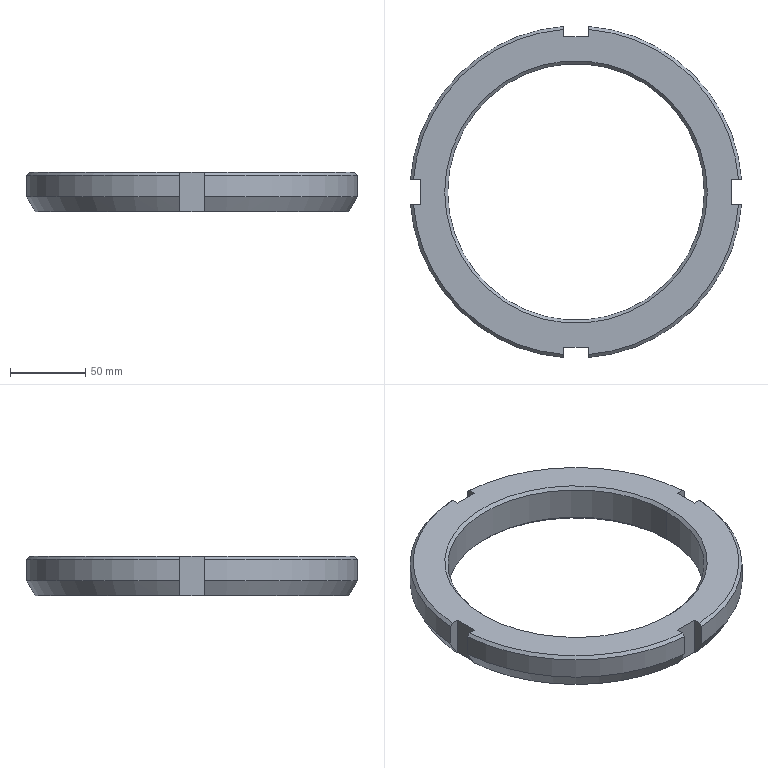Part | SolidWorks | features Chamfer 3, ICE 2, Extrusion 1 | 1 solid | 32 faces | box 219.417 x 219.417 x 26 mm | volume 365558 mm3 | plane 14 | cone 12 | cylinder 6 | commonest cylinder face diameters 220 x4 170 x2
STEP:
#1=CARTESIAN_POINT('',(85.,0.,2.));
#2=VERTEX_POINT('',#1);
#3=CARTESIAN_POINT('',(-85.,0.,2.));
#4=VERTEX_POINT('',#3);
#5=CARTESIAN_POINT('',(0.,0.,2.));
#6=DIRECTION('',(0.,0.,-1.));
#7=DIRECTION('',(1.,0.,0.));
#8=AXIS2_PLACEMENT_3D('',#5,#6,#7);
#9=CIRCLE('',#8,85.);
#10=EDGE_CURVE('',#2,#4,#9,.T.);
#11=ORIENTED_EDGE('',*,*,#10,.F.);
#12=CARTESIAN_POINT('',(87.,0.,0.));
#13=VERTEX_POINT('',#12);
#14=CARTESIAN_POINT('',(85.,0.,2.));
#15=DIRECTION('',(0.7071,0.,-0.7071));
#16=VECTOR('',#15,1000.);
#17=LINE('',#14,#16);
#18=EDGE_CURVE('',#2,#13,#17,.T.);
#19=ORIENTED_EDGE('',*,*,#18,.T.);
#20=CARTESIAN_POINT('',(-87.,0.,0.));
#21=VERTEX_POINT('',#20);
#22=CARTESIAN_POINT('',(0.,0.,0.));
#23=DIRECTION('',(0.,0.,1.));
#24=DIRECTION('',(1.,0.,0.));
#25=AXIS2_PLACEMENT_3D('',#22,#23,#24);
#26=CIRCLE('',#25,87.);
#27=EDGE_CURVE('',#21,#13,#26,.T.);
#28=ORIENTED_EDGE('',*,*,#27,.F.);
#29=CARTESIAN_POINT('',(-85.,0.,2.));
#30=DIRECTION('',(-0.7071,0.,-0.7071));
#31=VECTOR('',#30,1000.);
#32=LINE('',#29,#31);
#33=EDGE_CURVE('',#4,#21,#32,.T.);
#34=ORIENTED_EDGE('',*,*,#33,.F.);
#35=EDGE_LOOP('',(#11,#19,#28,#34));
#36=FACE_OUTER_BOUND('',#35,.T.);
#37=CARTESIAN_POINT('',(0.,0.,2.));
#38=DIRECTION('',(0.,0.,-1.));
#39=DIRECTION('',(-1.,0.,0.));
#40=AXIS2_PLACEMENT_3D('',#37,#38,#39);
#41=CONICAL_SURFACE('',#40,85.,0.7854);
#42=ADVANCED_FACE('',(#36),#41,.F.);
#43=CARTESIAN_POINT('',(-85.,0.,24.));
#44=VERTEX_POINT('',#43);
#45=CARTESIAN_POINT('',(85.,0.,24.));
#46=VERTEX_POINT('',#45);
#47=CARTESIAN_POINT('',(0.,0.,24.));
#48=DIRECTION('',(0.,0.,1.));
#49=DIRECTION('',(1.,0.,0.));
#50=AXIS2_PLACEMENT_3D('',#47,#48,#49);
#51=CIRCLE('',#50,85.);
#52=EDGE_CURVE('',#44,#46,#51,.T.);
#53=ORIENTED_EDGE('',*,*,#52,.F.);
#54=CARTESIAN_POINT('',(-87.,0.,26.));
#55=VERTEX_POINT('',#54);
#56=CARTESIAN_POINT('',(-87.,0.,26.));
#57=DIRECTION('',(-0.7071,0.,0.7071));
#58=VECTOR('',#57,1000.);
#59=LINE('',#56,#58);
#60=EDGE_CURVE('',#44,#55,#59,.T.);
#61=ORIENTED_EDGE('',*,*,#60,.T.);
#62=CARTESIAN_POINT('',(87.,0.,26.));
#63=VERTEX_POINT('',#62);
#64=CARTESIAN_POINT('',(0.,0.,26.));
#65=DIRECTION('',(0.,0.,-1.));
#66=DIRECTION('',(1.,0.,0.));
#67=AXIS2_PLACEMENT_3D('',#64,#65,#66);
#68=CIRCLE('',#67,87.);
#69=EDGE_CURVE('',#63,#55,#68,.T.);
#70=ORIENTED_EDGE('',*,*,#69,.F.);
#71=CARTESIAN_POINT('',(87.,0.,26.));
#72=DIRECTION('',(0.7071,0.,0.7071));
#73=VECTOR('',#72,1000.);
#74=LINE('',#71,#73);
#75=EDGE_CURVE('',#46,#63,#74,.T.);
#76=ORIENTED_EDGE('',*,*,#75,.F.);
#77=EDGE_LOOP('',(#53,#61,#70,#76));
#78=FACE_OUTER_BOUND('',#77,.T.);
#79=CARTESIAN_POINT('',(0.,0.,26.));
#80=DIRECTION('',(0.,0.,1.));
#81=DIRECTION('',(1.,0.,0.));
#82=AXIS2_PLACEMENT_3D('',#79,#80,#81);
#83=CONICAL_SURFACE('',#82,87.,0.7854);
#84=ADVANCED_FACE('',(#78),#83,.F.);
#85=ORIENTED_EDGE('',*,*,#52,.T.);
#86=CARTESIAN_POINT('',(85.,0.,26.));
#87=DIRECTION('',(0.,0.,-1.));
#88=VECTOR('',#87,1000.);
#89=LINE('',#86,#88);
#90=EDGE_CURVE('',#46,#2,#89,.T.);
#91=ORIENTED_EDGE('',*,*,#90,.T.);
#92=ORIENTED_EDGE('',*,*,#10,.T.);
#93=CARTESIAN_POINT('',(-85.,0.,26.));
#94=DIRECTION('',(0.,0.,-1.));
#95=VECTOR('',#94,1000.);
#96=LINE('',#93,#95);
#97=EDGE_CURVE('',#44,#4,#96,.T.);
#98=ORIENTED_EDGE('',*,*,#97,.F.);
#99=EDGE_LOOP('',(#85,#91,#92,#98));
#100=FACE_OUTER_BOUND('',#99,.T.);
#101=CARTESIAN_POINT('',(0.,0.,26.));
#102=DIRECTION('',(0.,0.,-1.));
#103=DIRECTION('',(-1.,0.,0.));
#104=AXIS2_PLACEMENT_3D('',#101,#102,#103);
#105=CYLINDRICAL_SURFACE('',#104,85.);
#106=ADVANCED_FACE('',(#100),#105,.F.);
#107=CARTESIAN_POINT('',(8.,-109.709,24.));
#108=VERTEX_POINT('',#107);
#109=CARTESIAN_POINT('',(8.,-109.709,10.));
#110=VERTEX_POINT('',#109);
#111=CARTESIAN_POINT('',(8.,-109.709,26.));
#112=DIRECTION('',(0.,0.,-1.));
#113=VECTOR('',#112,1000.);
#114=LINE('',#111,#113);
#115=EDGE_CURVE('',#108,#110,#114,.T.);
#116=ORIENTED_EDGE('',*,*,#115,.T.);
#117=CARTESIAN_POINT('',(109.709,-8.,10.));
#118=VERTEX_POINT('',#117);
#119=CARTESIAN_POINT('',(0.,0.,10.));
#120=DIRECTION('',(0.,0.,1.));
#121=DIRECTION('',(1.,0.,0.));
#122=AXIS2_PLACEMENT_3D('',#119,#120,#121);
#123=CIRCLE('',#122,110.);
#124=EDGE_CURVE('',#110,#118,#123,.T.);
#125=ORIENTED_EDGE('',*,*,#124,.T.);
#126=CARTESIAN_POINT('',(109.709,-8.,24.));
#127=VERTEX_POINT('',#126);
#128=CARTESIAN_POINT('',(109.709,-8.,26.));
#129=DIRECTION('',(0.,0.,1.));
#130=VECTOR('',#129,1000.);
#131=LINE('',#128,#130);
#132=EDGE_CURVE('',#118,#127,#131,.T.);
#133=ORIENTED_EDGE('',*,*,#132,.T.);
#134=CARTESIAN_POINT('',(0.,0.,24.));
#135=DIRECTION('',(0.,0.,-1.));
#136=DIRECTION('',(1.,0.,0.));
#137=AXIS2_PLACEMENT_3D('',#134,#135,#136);
#138=CIRCLE('',#137,110.);
#139=EDGE_CURVE('',#127,#108,#138,.T.);
#140=ORIENTED_EDGE('',*,*,#139,.T.);
#141=EDGE_LOOP('',(#116,#125,#133,#140));
#142=FACE_OUTER_BOUND('',#141,.T.);
#143=CARTESIAN_POINT('',(0.,0.,26.));
#144=DIRECTION('',(0.,0.,-1.));
#145=DIRECTION('',(-1.,0.,0.));
#146=AXIS2_PLACEMENT_3D('',#143,#144,#145);
#147=CYLINDRICAL_SURFACE('',#146,110.);
#148=ADVANCED_FACE('',(#142),#147,.T.);
#149=CARTESIAN_POINT('',(-8.,109.709,24.));
#150=VERTEX_POINT('',#149);
#151=CARTESIAN_POINT('',(-8.,109.709,10.));
#152=VERTEX_POINT('',#151);
#153=CARTESIAN_POINT('',(-8.,109.709,26.));
#154=DIRECTION('',(0.,0.,-1.));
#155=VECTOR('',#154,1000.);
#156=LINE('',#153,#155);
#157=EDGE_CURVE('',#150,#152,#156,.T.);
#158=ORIENTED_EDGE('',*,*,#157,.T.);
#159=CARTESIAN_POINT('',(-109.709,8.,10.));
#160=VERTEX_POINT('',#159);
#161=CARTESIAN_POINT('',(0.,0.,10.));
#162=DIRECTION('',(0.,0.,1.));
#163=DIRECTION('',(1.,0.,0.));
#164=AXIS2_PLACEMENT_3D('',#161,#162,#163);
#165=CIRCLE('',#164,110.);
#166=EDGE_CURVE('',#152,#160,#165,.T.);
#167=ORIENTED_EDGE('',*,*,#166,.T.);
#168=CARTESIAN_POINT('',(-109.709,8.,24.));
#169=VERTEX_POINT('',#168);
#170=CARTESIAN_POINT('',(-109.709,8.,26.));
#171=DIRECTION('',(0.,0.,1.));
#172=VECTOR('',#171,1000.);
#173=LINE('',#170,#172);
#174=EDGE_CURVE('',#160,#169,#173,.T.);
#175=ORIENTED_EDGE('',*,*,#174,.T.);
#176=CARTESIAN_POINT('',(0.,0.,24.));
#177=DIRECTION('',(0.,0.,-1.));
#178=DIRECTION('',(1.,0.,0.));
#179=AXIS2_PLACEMENT_3D('',#176,#177,#178);
#180=CIRCLE('',#179,110.);
#181=EDGE_CURVE('',#169,#150,#180,.T.);
#182=ORIENTED_EDGE('',*,*,#181,.T.);
#183=EDGE_LOOP('',(#158,#167,#175,#182));
#184=FACE_OUTER_BOUND('',#183,.T.);
#185=CARTESIAN_POINT('',(0.,0.,26.));
#186=DIRECTION('',(0.,0.,-1.));
#187=DIRECTION('',(-1.,0.,0.));
#188=AXIS2_PLACEMENT_3D('',#185,#186,#187);
#189=CYLINDRICAL_SURFACE('',#188,110.);
#190=ADVANCED_FACE('',(#184),#189,.T.);
#191=CARTESIAN_POINT('',(-109.709,-8.,24.));
#192=VERTEX_POINT('',#191);
#193=CARTESIAN_POINT('',(-109.709,-8.,10.));
#194=VERTEX_POINT('',#193);
#195=CARTESIAN_POINT('',(-109.709,-8.,26.));
#196=DIRECTION('',(0.,0.,-1.));
#197=VECTOR('',#196,1000.);
#198=LINE('',#195,#197);
#199=EDGE_CURVE('',#192,#194,#198,.T.);
#200=ORIENTED_EDGE('',*,*,#199,.T.);
#201=CARTESIAN_POINT('',(-8.,-109.709,10.));
#202=VERTEX_POINT('',#201);
#203=CARTESIAN_POINT('',(0.,0.,10.));
#204=DIRECTION('',(0.,0.,1.));
#205=DIRECTION('',(1.,0.,0.));
#206=AXIS2_PLACEMENT_3D('',#203,#204,#205);
#207=CIRCLE('',#206,110.);
#208=EDGE_CURVE('',#194,#202,#207,.T.);
#209=ORIENTED_EDGE('',*,*,#208,.T.);
#210=CARTESIAN_POINT('',(-8.,-109.709,24.));
#211=VERTEX_POINT('',#210);
#212=CARTESIAN_POINT('',(-8.,-109.709,26.));
#213=DIRECTION('',(0.,0.,1.));
#214=VECTOR('',#213,1000.);
#215=LINE('',#212,#214);
#216=EDGE_CURVE('',#202,#211,#215,.T.);
#217=ORIENTED_EDGE('',*,*,#216,.T.);
#218=CARTESIAN_POINT('',(0.,0.,24.));
#219=DIRECTION('',(0.,0.,-1.));
#220=DIRECTION('',(1.,0.,0.));
#221=AXIS2_PLACEMENT_3D('',#218,#219,#220);
#222=CIRCLE('',#221,110.);
#223=EDGE_CURVE('',#211,#192,#222,.T.);
#224=ORIENTED_EDGE('',*,*,#223,.T.);
#225=EDGE_LOOP('',(#200,#209,#217,#224));
#226=FACE_OUTER_BOUND('',#225,.T.);
#227=CARTESIAN_POINT('',(0.,0.,26.));
#228=DIRECTION('',(0.,0.,-1.));
#229=DIRECTION('',(-1.,0.,0.));
#230=AXIS2_PLACEMENT_3D('',#227,#228,#229);
#231=CYLINDRICAL_SURFACE('',#230,110.);
#232=ADVANCED_FACE('',(#226),#231,.T.);
#233=CARTESIAN_POINT('',(109.709,8.,24.));
#234=VERTEX_POINT('',#233);
#235=CARTESIAN_POINT('',(109.709,8.,10.));
#236=VERTEX_POINT('',#235);
#237=CARTESIAN_POINT('',(109.709,8.,26.));
#238=DIRECTION('',(0.,0.,-1.));
#239=VECTOR('',#238,1000.);
#240=LINE('',#237,#239);
#241=EDGE_CURVE('',#234,#236,#240,.T.);
#242=ORIENTED_EDGE('',*,*,#241,.T.);
#243=CARTESIAN_POINT('',(8.,109.709,10.));
#244=VERTEX_POINT('',#243);
#245=CARTESIAN_POINT('',(0.,0.,10.));
#246=DIRECTION('',(0.,0.,1.));
#247=DIRECTION('',(1.,0.,0.));
#248=AXIS2_PLACEMENT_3D('',#245,#246,#247);
#249=CIRCLE('',#248,110.);
#250=EDGE_CURVE('',#236,#244,#249,.T.);
#251=ORIENTED_EDGE('',*,*,#250,.T.);
#252=CARTESIAN_POINT('',(8.,109.709,24.));
#253=VERTEX_POINT('',#252);
#254=CARTESIAN_POINT('',(8.,109.709,26.));
#255=DIRECTION('',(0.,0.,1.));
#256=VECTOR('',#255,1000.);
#257=LINE('',#254,#256);
#258=EDGE_CURVE('',#244,#253,#257,.T.);
#259=ORIENTED_EDGE('',*,*,#258,.T.);
#260=CARTESIAN_POINT('',(0.,0.,24.));
#261=DIRECTION('',(0.,0.,-1.));
#262=DIRECTION('',(1.,0.,0.));
#263=AXIS2_PLACEMENT_3D('',#260,#261,#262);
#264=CIRCLE('',#263,110.);
#265=EDGE_CURVE('',#253,#234,#264,.T.);
#266=ORIENTED_EDGE('',*,*,#265,.T.);
#267=EDGE_LOOP('',(#242,#251,#259,#266));
#268=FACE_OUTER_BOUND('',#267,.T.);
#269=CARTESIAN_POINT('',(0.,0.,26.));
#270=DIRECTION('',(0.,0.,-1.));
#271=DIRECTION('',(-1.,0.,0.));
#272=AXIS2_PLACEMENT_3D('',#269,#270,#271);
#273=CYLINDRICAL_SURFACE('',#272,110.);
#274=ADVANCED_FACE('',(#268),#273,.T.);
#275=ORIENTED_EDGE('',*,*,#69,.T.);
#276=CARTESIAN_POINT('',(0.,0.,26.));
#277=DIRECTION('',(0.,0.,-1.));
#278=DIRECTION('',(1.,0.,0.));
#279=AXIS2_PLACEMENT_3D('',#276,#277,#278);
#280=CIRCLE('',#279,87.);
#281=EDGE_CURVE('',#55,#63,#280,.T.);
#282=ORIENTED_EDGE('',*,*,#281,.T.);
#283=EDGE_LOOP('',(#275,#282));
#284=FACE_BOUND('',#283,.T.);
#285=CARTESIAN_POINT('',(8.,-107.703,26.));
#286=VERTEX_POINT('',#285);
#287=CARTESIAN_POINT('',(8.,-103.,26.));
#288=VERTEX_POINT('',#287);
#289=CARTESIAN_POINT('',(8.,-103.,26.));
#290=DIRECTION('',(0.,1.,0.));
#291=VECTOR('',#290,1000.);
#292=LINE('',#289,#291);
#293=EDGE_CURVE('',#286,#288,#292,.T.);
#294=ORIENTED_EDGE('',*,*,#293,.F.);
#295=CARTESIAN_POINT('',(107.703,-8.,26.));
#296=VERTEX_POINT('',#295);
#297=CARTESIAN_POINT('',(0.,0.,26.));
#298=DIRECTION('',(0.,0.,1.));
#299=DIRECTION('',(1.,0.,0.));
#300=AXIS2_PLACEMENT_3D('',#297,#298,#299);
#301=CIRCLE('',#300,108.);
#302=EDGE_CURVE('',#286,#296,#301,.T.);
#303=ORIENTED_EDGE('',*,*,#302,.T.);
#304=CARTESIAN_POINT('',(103.,-8.,26.));
#305=VERTEX_POINT('',#304);
#306=CARTESIAN_POINT('',(103.,-8.,26.));
#307=DIRECTION('',(1.,0.,0.));
#308=VECTOR('',#307,1000.);
#309=LINE('',#306,#308);
#310=EDGE_CURVE('',#305,#296,#309,.T.);
#311=ORIENTED_EDGE('',*,*,#310,.F.);
#312=CARTESIAN_POINT('',(103.,8.,26.));
#313=VERTEX_POINT('',#312);
#314=CARTESIAN_POINT('',(103.,8.,26.));
#315=DIRECTION('',(0.,-1.,0.));
#316=VECTOR('',#315,1000.);
#317=LINE('',#314,#316);
#318=EDGE_CURVE('',#313,#305,#317,.T.);
#319=ORIENTED_EDGE('',*,*,#318,.F.);
#320=CARTESIAN_POINT('',(107.703,8.,26.));
#321=VERTEX_POINT('',#320);
#322=CARTESIAN_POINT('',(103.,8.,26.));
#323=DIRECTION('',(-1.,0.,0.));
#324=VECTOR('',#323,1000.);
#325=LINE('',#322,#324);
#326=EDGE_CURVE('',#321,#313,#325,.T.);
#327=ORIENTED_EDGE('',*,*,#326,.F.);
#328=CARTESIAN_POINT('',(8.,107.703,26.));
#329=VERTEX_POINT('',#328);
#330=CARTESIAN_POINT('',(0.,0.,26.));
#331=DIRECTION('',(0.,0.,1.));
#332=DIRECTION('',(1.,0.,0.));
#333=AXIS2_PLACEMENT_3D('',#330,#331,#332);
#334=CIRCLE('',#333,108.);
#335=EDGE_CURVE('',#321,#329,#334,.T.);
#336=ORIENTED_EDGE('',*,*,#335,.T.);
#337=CARTESIAN_POINT('',(8.,103.,26.));
#338=VERTEX_POINT('',#337);
#339=CARTESIAN_POINT('',(8.,109.954,26.));
#340=DIRECTION('',(0.,1.,0.));
#341=VECTOR('',#340,1000.);
#342=LINE('',#339,#341);
#343=EDGE_CURVE('',#338,#329,#342,.T.);
#344=ORIENTED_EDGE('',*,*,#343,.F.);
#345=CARTESIAN_POINT('',(-8.,103.,26.));
#346=VERTEX_POINT('',#345);
#347=CARTESIAN_POINT('',(-8.,103.,26.));
#348=DIRECTION('',(1.,0.,0.));
#349=VECTOR('',#348,1000.);
#350=LINE('',#347,#349);
#351=EDGE_CURVE('',#346,#338,#350,.T.);
#352=ORIENTED_EDGE('',*,*,#351,.F.);
#353=CARTESIAN_POINT('',(-8.,107.703,26.));
#354=VERTEX_POINT('',#353);
#355=CARTESIAN_POINT('',(-8.,109.954,26.));
#356=DIRECTION('',(0.,-1.,0.));
#357=VECTOR('',#356,1000.);
#358=LINE('',#355,#357);
#359=EDGE_CURVE('',#354,#346,#358,.T.);
#360=ORIENTED_EDGE('',*,*,#359,.F.);
#361=CARTESIAN_POINT('',(-107.703,8.,26.));
#362=VERTEX_POINT('',#361);
#363=CARTESIAN_POINT('',(0.,0.,26.));
#364=DIRECTION('',(0.,0.,1.));
#365=DIRECTION('',(1.,0.,0.));
#366=AXIS2_PLACEMENT_3D('',#363,#364,#365);
#367=CIRCLE('',#366,108.);
#368=EDGE_CURVE('',#354,#362,#367,.T.);
#369=ORIENTED_EDGE('',*,*,#368,.T.);
#370=CARTESIAN_POINT('',(-103.,8.,26.));
#371=VERTEX_POINT('',#370);
#372=CARTESIAN_POINT('',(-109.954,8.,26.));
#373=DIRECTION('',(-1.,0.,0.));
#374=VECTOR('',#373,1000.);
#375=LINE('',#372,#374);
#376=EDGE_CURVE('',#371,#362,#375,.T.);
#377=ORIENTED_EDGE('',*,*,#376,.F.);
#378=CARTESIAN_POINT('',(-103.,-8.,26.));
#379=VERTEX_POINT('',#378);
#380=CARTESIAN_POINT('',(-103.,8.,26.));
#381=DIRECTION('',(0.,1.,0.));
#382=VECTOR('',#381,1000.);
#383=LINE('',#380,#382);
#384=EDGE_CURVE('',#379,#371,#383,.T.);
#385=ORIENTED_EDGE('',*,*,#384,.F.);
#386=CARTESIAN_POINT('',(-107.703,-8.,26.));
#387=VERTEX_POINT('',#386);
#388=CARTESIAN_POINT('',(-109.954,-8.,26.));
#389=DIRECTION('',(1.,0.,0.));
#390=VECTOR('',#389,1000.);
#391=LINE('',#388,#390);
#392=EDGE_CURVE('',#387,#379,#391,.T.);
#393=ORIENTED_EDGE('',*,*,#392,.F.);
#394=CARTESIAN_POINT('',(-8.,-107.703,26.));
#395=VERTEX_POINT('',#394);
#396=CARTESIAN_POINT('',(0.,0.,26.));
#397=DIRECTION('',(0.,0.,1.));
#398=DIRECTION('',(1.,0.,0.));
#399=AXIS2_PLACEMENT_3D('',#396,#397,#398);
#400=CIRCLE('',#399,108.);
#401=EDGE_CURVE('',#387,#395,#400,.T.);
#402=ORIENTED_EDGE('',*,*,#401,.T.);
#403=CARTESIAN_POINT('',(-8.,-103.,26.));
#404=VERTEX_POINT('',#403);
#405=CARTESIAN_POINT('',(-8.,-103.,26.));
#406=DIRECTION('',(0.,-1.,0.));
#407=VECTOR('',#406,1000.);
#408=LINE('',#405,#407);
#409=EDGE_CURVE('',#404,#395,#408,.T.);
#410=ORIENTED_EDGE('',*,*,#409,.F.);
#411=CARTESIAN_POINT('',(-8.,-103.,26.));
#412=DIRECTION('',(-1.,0.,0.));
#413=VECTOR('',#412,1000.);
#414=LINE('',#411,#413);
#415=EDGE_CURVE('',#288,#404,#414,.T.);
#416=ORIENTED_EDGE('',*,*,#415,.F.);
#417=EDGE_LOOP('',(#294,#303,#311,#319,#327,#336,#344,#352,#360,#369,#377,#385,#393,#402,#410,#416));
#418=FACE_OUTER_BOUND('',#417,.T.);
#419=CARTESIAN_POINT('',(0.,0.,26.));
#420=DIRECTION('',(0.,0.,1.));
#421=DIRECTION('',(1.,0.,0.));
#422=AXIS2_PLACEMENT_3D('',#419,#420,#421);
#423=PLANE('',#422);
#424=ADVANCED_FACE('',(#284,#418),#423,.T.);
#425=ORIENTED_EDGE('',*,*,#27,.T.);
#426=CARTESIAN_POINT('',(0.,0.,0.));
#427=DIRECTION('',(0.,0.,1.));
#428=DIRECTION('',(1.,0.,0.));
#429=AXIS2_PLACEMENT_3D('',#426,#427,#428);
#430=CIRCLE('',#429,87.);
#431=EDGE_CURVE('',#13,#21,#430,.T.);
#432=ORIENTED_EDGE('',*,*,#431,.T.);
#433=EDGE_LOOP('',(#425,#432));
#434=FACE_BOUND('',#433,.T.);
#435=CARTESIAN_POINT('',(-8.,-103.,0.));
#436=VERTEX_POINT('',#435);
#437=CARTESIAN_POINT('',(-8.,-103.919,0.));
#438=VERTEX_POINT('',#437);
#439=CARTESIAN_POINT('',(-8.,-103.,0.));
#440=DIRECTION('',(0.,-1.,0.));
#441=VECTOR('',#440,1000.);
#442=LINE('',#439,#441);
#443=EDGE_CURVE('',#436,#438,#442,.T.);
#444=ORIENTED_EDGE('',*,*,#443,.T.);
#445=CARTESIAN_POINT('',(-103.919,-8.,0.));
#446=VERTEX_POINT('',#445);
#447=CARTESIAN_POINT('',(0.,0.,0.));
#448=DIRECTION('',(0.,0.,-1.));
#449=DIRECTION('',(1.,0.,0.));
#450=AXIS2_PLACEMENT_3D('',#447,#448,#449);
#451=CIRCLE('',#450,104.226);
#452=EDGE_CURVE('',#438,#446,#451,.T.);
#453=ORIENTED_EDGE('',*,*,#452,.T.);
#454=CARTESIAN_POINT('',(-103.,-8.,0.));
#455=VERTEX_POINT('',#454);
#456=CARTESIAN_POINT('',(0.,-8.,0.));
#457=DIRECTION('',(1.,0.,0.));
#458=VECTOR('',#457,1000.);
#459=LINE('',#456,#458);
#460=EDGE_CURVE('',#446,#455,#459,.T.);
#461=ORIENTED_EDGE('',*,*,#460,.T.);
#462=CARTESIAN_POINT('',(-103.,8.,0.));
#463=VERTEX_POINT('',#462);
#464=CARTESIAN_POINT('',(-103.,8.,0.));
#465=DIRECTION('',(0.,1.,0.));
#466=VECTOR('',#465,1000.);
#467=LINE('',#464,#466);
#468=EDGE_CURVE('',#455,#463,#467,.T.);
#469=ORIENTED_EDGE('',*,*,#468,.T.);
#470=CARTESIAN_POINT('',(-103.919,8.,0.));
#471=VERTEX_POINT('',#470);
#472=CARTESIAN_POINT('',(-109.954,8.,0.));
#473=DIRECTION('',(-1.,0.,0.));
#474=VECTOR('',#473,1000.);
#475=LINE('',#472,#474);
#476=EDGE_CURVE('',#463,#471,#475,.T.);
#477=ORIENTED_EDGE('',*,*,#476,.T.);
#478=CARTESIAN_POINT('',(-8.,103.919,0.));
#479=VERTEX_POINT('',#478);
#480=CARTESIAN_POINT('',(0.,0.,0.));
#481=DIRECTION('',(0.,0.,-1.));
#482=DIRECTION('',(1.,0.,0.));
#483=AXIS2_PLACEMENT_3D('',#480,#481,#482);
#484=CIRCLE('',#483,104.226);
#485=EDGE_CURVE('',#471,#479,#484,.T.);
#486=ORIENTED_EDGE('',*,*,#485,.T.);
#487=CARTESIAN_POINT('',(-8.,103.,0.));
#488=VERTEX_POINT('',#487);
#489=CARTESIAN_POINT('',(-8.,0.,0.));
#490=DIRECTION('',(0.,-1.,0.));
#491=VECTOR('',#490,1000.);
#492=LINE('',#489,#491);
#493=EDGE_CURVE('',#479,#488,#492,.T.);
#494=ORIENTED_EDGE('',*,*,#493,.T.);
#495=CARTESIAN_POINT('',(8.,103.,0.));
#496=VERTEX_POINT('',#495);
#497=CARTESIAN_POINT('',(-8.,103.,0.));
#498=DIRECTION('',(1.,0.,0.));
#499=VECTOR('',#498,1000.);
#500=LINE('',#497,#499);
#501=EDGE_CURVE('',#488,#496,#500,.T.);
#502=ORIENTED_EDGE('',*,*,#501,.T.);
#503=CARTESIAN_POINT('',(8.,103.919,0.));
#504=VERTEX_POINT('',#503);
#505=CARTESIAN_POINT('',(8.,109.954,0.));
#506=DIRECTION('',(0.,1.,0.));
#507=VECTOR('',#506,1000.);
#508=LINE('',#505,#507);
#509=EDGE_CURVE('',#496,#504,#508,.T.);
#510=ORIENTED_EDGE('',*,*,#509,.T.);
#511=CARTESIAN_POINT('',(103.919,8.,0.));
#512=VERTEX_POINT('',#511);
#513=CARTESIAN_POINT('',(0.,0.,0.));
#514=DIRECTION('',(0.,0.,-1.));
#515=DIRECTION('',(1.,0.,0.));
#516=AXIS2_PLACEMENT_3D('',#513,#514,#515);
#517=CIRCLE('',#516,104.226);
#518=EDGE_CURVE('',#504,#512,#517,.T.);
#519=ORIENTED_EDGE('',*,*,#518,.T.);
#520=CARTESIAN_POINT('',(103.,8.,0.));
#521=VERTEX_POINT('',#520);
#522=CARTESIAN_POINT('',(0.,8.,0.));
#523=DIRECTION('',(-1.,0.,0.));
#524=VECTOR('',#523,1000.);
#525=LINE('',#522,#524);
#526=EDGE_CURVE('',#512,#521,#525,.T.);
#527=ORIENTED_EDGE('',*,*,#526,.T.);
#528=CARTESIAN_POINT('',(103.,-8.,0.));
#529=VERTEX_POINT('',#528);
#530=CARTESIAN_POINT('',(103.,8.,0.));
#531=DIRECTION('',(0.,-1.,0.));
#532=VECTOR('',#531,1000.);
#533=LINE('',#530,#532);
#534=EDGE_CURVE('',#521,#529,#533,.T.);
#535=ORIENTED_EDGE('',*,*,#534,.T.);
#536=CARTESIAN_POINT('',(103.919,-8.,0.));
#537=VERTEX_POINT('',#536);
#538=CARTESIAN_POINT('',(103.,-8.,0.));
#539=DIRECTION('',(1.,0.,0.));
#540=VECTOR('',#539,1000.);
#541=LINE('',#538,#540);
#542=EDGE_CURVE('',#529,#537,#541,.T.);
#543=ORIENTED_EDGE('',*,*,#542,.T.);
#544=CARTESIAN_POINT('',(8.,-103.919,0.));
#545=VERTEX_POINT('',#544);
#546=CARTESIAN_POINT('',(0.,0.,0.));
#547=DIRECTION('',(0.,0.,-1.));
#548=DIRECTION('',(1.,0.,0.));
#549=AXIS2_PLACEMENT_3D('',#546,#547,#548);
#550=CIRCLE('',#549,104.226);
#551=EDGE_CURVE('',#537,#545,#550,.T.);
#552=ORIENTED_EDGE('',*,*,#551,.T.);
#553=CARTESIAN_POINT('',(8.,-103.,0.));
#554=VERTEX_POINT('',#553);
#555=CARTESIAN_POINT('',(8.,0.,0.));
#556=DIRECTION('',(0.,1.,0.));
#557=VECTOR('',#556,1000.);
#558=LINE('',#555,#557);
#559=EDGE_CURVE('',#545,#554,#558,.T.);
#560=ORIENTED_EDGE('',*,*,#559,.T.);
#561=CARTESIAN_POINT('',(-8.,-103.,0.));
#562=DIRECTION('',(-1.,0.,0.));
#563=VECTOR('',#562,1000.);
#564=LINE('',#561,#563);
#565=EDGE_CURVE('',#554,#436,#564,.T.);
#566=ORIENTED_EDGE('',*,*,#565,.T.);
#567=EDGE_LOOP('',(#444,#453,#461,#469,#477,#486,#494,#502,#510,#519,#527,#535,#543,#552,#560,#566));
#568=FACE_OUTER_BOUND('',#567,.T.);
#569=CARTESIAN_POINT('',(0.,0.,0.));
#570=DIRECTION('',(0.,0.,1.));
#571=DIRECTION('',(1.,0.,0.));
#572=AXIS2_PLACEMENT_3D('',#569,#570,#571);
#573=PLANE('',#572);
#574=ADVANCED_FACE('',(#434,#568),#573,.F.);
#575=ORIENTED_EDGE('',*,*,#526,.F.);
#576=CARTESIAN_POINT('',(103.919,8.,0.));
#577=CARTESIAN_POINT('',(105.849,8.,3.333));
#578=CARTESIAN_POINT('',(107.779,8.,6.667));
#579=CARTESIAN_POINT('',(109.709,8.,10.));
#580=B_SPLINE_CURVE_WITH_KNOTS('',3,(#576,#577,#578,#579),.UNSPECIFIED.,.F.,.F.,(4,4),(0.,0.01156),.UNSPECIFIED.);
#581=EDGE_CURVE('',#512,#236,#580,.T.);
#582=ORIENTED_EDGE('',*,*,#581,.T.);
#583=ORIENTED_EDGE('',*,*,#241,.F.);
#584=CARTESIAN_POINT('',(109.709,8.,24.));
#585=CARTESIAN_POINT('',(109.04,8.,24.667));
#586=CARTESIAN_POINT('',(108.372,8.,25.333));
#587=CARTESIAN_POINT('',(107.703,8.,26.));
#588=B_SPLINE_CURVE_WITH_KNOTS('',3,(#584,#585,#586,#587),.UNSPECIFIED.,.F.,.F.,(4,4),(0.,0.002832),.UNSPECIFIED.);
#589=EDGE_CURVE('',#234,#321,#588,.T.);
#590=ORIENTED_EDGE('',*,*,#589,.T.);
#591=ORIENTED_EDGE('',*,*,#326,.T.);
#592=CARTESIAN_POINT('',(103.,8.,0.));
#593=DIRECTION('',(0.,0.,1.));
#594=VECTOR('',#593,1000.);
#595=LINE('',#592,#594);
#596=EDGE_CURVE('',#521,#313,#595,.T.);
#597=ORIENTED_EDGE('',*,*,#596,.F.);
#598=EDGE_LOOP('',(#575,#582,#583,#590,#591,#597));
#599=FACE_OUTER_BOUND('',#598,.T.);
#600=CARTESIAN_POINT('',(103.,8.,0.));
#601=DIRECTION('',(0.,1.,0.));
#602=DIRECTION('',(0.,0.,1.));
#603=AXIS2_PLACEMENT_3D('',#600,#601,#602);
#604=PLANE('',#603);
#605=ADVANCED_FACE('',(#599),#604,.F.);
#606=ORIENTED_EDGE('',*,*,#132,.F.);
#607=CARTESIAN_POINT('',(109.709,-8.,10.));
#608=CARTESIAN_POINT('',(107.779,-8.,6.667));
#609=CARTESIAN_POINT('',(105.849,-8.,3.333));
#610=CARTESIAN_POINT('',(103.919,-8.,0.));
#611=B_SPLINE_CURVE_WITH_KNOTS('',3,(#607,#608,#609,#610),.UNSPECIFIED.,.F.,.F.,(4,4),(0.,0.01156),.UNSPECIFIED.);
#612=EDGE_CURVE('',#118,#537,#611,.T.);
#613=ORIENTED_EDGE('',*,*,#612,.T.);
#614=ORIENTED_EDGE('',*,*,#542,.F.);
#615=CARTESIAN_POINT('',(103.,-8.,0.));
#616=DIRECTION('',(0.,0.,1.));
#617=VECTOR('',#616,1000.);
#618=LINE('',#615,#617);
#619=EDGE_CURVE('',#529,#305,#618,.T.);
#620=ORIENTED_EDGE('',*,*,#619,.T.);
#621=ORIENTED_EDGE('',*,*,#310,.T.);
#622=CARTESIAN_POINT('',(107.703,-8.,26.));
#623=CARTESIAN_POINT('',(108.372,-8.,25.333));
#624=CARTESIAN_POINT('',(109.04,-8.,24.667));
#625=CARTESIAN_POINT('',(109.709,-8.,24.));
#626=B_SPLINE_CURVE_WITH_KNOTS('',3,(#622,#623,#624,#625),.UNSPECIFIED.,.F.,.F.,(4,4),(0.,0.002832),.UNSPECIFIED.);
#627=EDGE_CURVE('',#296,#127,#626,.T.);
#628=ORIENTED_EDGE('',*,*,#627,.T.);
#629=EDGE_LOOP('',(#606,#613,#614,#620,#621,#628));
#630=FACE_OUTER_BOUND('',#629,.T.);
#631=CARTESIAN_POINT('',(103.,-8.,0.));
#632=DIRECTION('',(0.,-1.,0.));
#633=DIRECTION('',(0.,0.,-1.));
#634=AXIS2_PLACEMENT_3D('',#631,#632,#633);
#635=PLANE('',#634);
#636=ADVANCED_FACE('',(#630),#635,.F.);
#637=ORIENTED_EDGE('',*,*,#318,.T.);
#638=ORIENTED_EDGE('',*,*,#619,.F.);
#639=ORIENTED_EDGE('',*,*,#534,.F.);
#640=ORIENTED_EDGE('',*,*,#596,.T.);
#641=EDGE_LOOP('',(#637,#638,#639,#640));
#642=FACE_OUTER_BOUND('',#641,.T.);
#643=CARTESIAN_POINT('',(103.,8.,0.));
#644=DIRECTION('',(-1.,0.,0.));
#645=DIRECTION('',(0.,0.,1.));
#646=AXIS2_PLACEMENT_3D('',#643,#644,#645);
#647=PLANE('',#646);
#648=ADVANCED_FACE('',(#642),#647,.F.);
#649=ORIENTED_EDGE('',*,*,#493,.F.);
#650=CARTESIAN_POINT('',(-8.,103.919,0.));
#651=CARTESIAN_POINT('',(-8.,105.849,3.333));
#652=CARTESIAN_POINT('',(-8.,107.779,6.667));
#653=CARTESIAN_POINT('',(-8.,109.709,10.));
#654=B_SPLINE_CURVE_WITH_KNOTS('',3,(#650,#651,#652,#653),.UNSPECIFIED.,.F.,.F.,(4,4),(0.,0.01156),.UNSPECIFIED.);
#655=EDGE_CURVE('',#479,#152,#654,.T.);
#656=ORIENTED_EDGE('',*,*,#655,.T.);
#657=ORIENTED_EDGE('',*,*,#157,.F.);
#658=CARTESIAN_POINT('',(-8.,109.709,24.));
#659=CARTESIAN_POINT('',(-8.,109.04,24.667));
#660=CARTESIAN_POINT('',(-8.,108.372,25.333));
#661=CARTESIAN_POINT('',(-8.,107.703,26.));
#662=B_SPLINE_CURVE_WITH_KNOTS('',3,(#658,#659,#660,#661),.UNSPECIFIED.,.F.,.F.,(4,4),(0.,0.002832),.UNSPECIFIED.);
#663=EDGE_CURVE('',#150,#354,#662,.T.);
#664=ORIENTED_EDGE('',*,*,#663,.T.);
#665=ORIENTED_EDGE('',*,*,#359,.T.);
#666=CARTESIAN_POINT('',(-8.,103.,0.));
#667=DIRECTION('',(0.,0.,1.));
#668=VECTOR('',#667,1000.);
#669=LINE('',#666,#668);
#670=EDGE_CURVE('',#488,#346,#669,.T.);
#671=ORIENTED_EDGE('',*,*,#670,.F.);
#672=EDGE_LOOP('',(#649,#656,#657,#664,#665,#671));
#673=FACE_OUTER_BOUND('',#672,.T.);
#674=CARTESIAN_POINT('',(-8.,109.954,0.));
#675=DIRECTION('',(-1.,0.,0.));
#676=DIRECTION('',(0.,0.,1.));
#677=AXIS2_PLACEMENT_3D('',#674,#675,#676);
#678=PLANE('',#677);
#679=ADVANCED_FACE('',(#673),#678,.F.);
#680=ORIENTED_EDGE('',*,*,#258,.F.);
#681=CARTESIAN_POINT('',(8.,109.709,10.));
#682=CARTESIAN_POINT('',(8.,107.779,6.667));
#683=CARTESIAN_POINT('',(8.,105.849,3.333));
#684=CARTESIAN_POINT('',(8.,103.919,0.));
#685=B_SPLINE_CURVE_WITH_KNOTS('',3,(#681,#682,#683,#684),.UNSPECIFIED.,.F.,.F.,(4,4),(0.,0.01156),.UNSPECIFIED.);
#686=EDGE_CURVE('',#244,#504,#685,.T.);
#687=ORIENTED_EDGE('',*,*,#686,.T.);
#688=ORIENTED_EDGE('',*,*,#509,.F.);
#689=CARTESIAN_POINT('',(8.,103.,0.));
#690=DIRECTION('',(0.,0.,1.));
#691=VECTOR('',#690,1000.);
#692=LINE('',#689,#691);
#693=EDGE_CURVE('',#496,#338,#692,.T.);
#694=ORIENTED_EDGE('',*,*,#693,.T.);
#695=ORIENTED_EDGE('',*,*,#343,.T.);
#696=CARTESIAN_POINT('',(8.,107.703,26.));
#697=CARTESIAN_POINT('',(8.,108.372,25.333));
#698=CARTESIAN_POINT('',(8.,109.04,24.667));
#699=CARTESIAN_POINT('',(8.,109.709,24.));
#700=B_SPLINE_CURVE_WITH_KNOTS('',3,(#696,#697,#698,#699),.UNSPECIFIED.,.F.,.F.,(4,4),(0.,0.002832),.UNSPECIFIED.);
#701=EDGE_CURVE('',#329,#253,#700,.T.);
#702=ORIENTED_EDGE('',*,*,#701,.T.);
#703=EDGE_LOOP('',(#680,#687,#688,#694,#695,#702));
#704=FACE_OUTER_BOUND('',#703,.T.);
#705=CARTESIAN_POINT('',(8.,109.954,0.));
#706=DIRECTION('',(1.,0.,0.));
#707=DIRECTION('',(0.,0.,-1.));
#708=AXIS2_PLACEMENT_3D('',#705,#706,#707);
#709=PLANE('',#708);
#710=ADVANCED_FACE('',(#704),#709,.F.);
#711=ORIENTED_EDGE('',*,*,#351,.T.);
#712=ORIENTED_EDGE('',*,*,#693,.F.);
#713=ORIENTED_EDGE('',*,*,#501,.F.);
#714=ORIENTED_EDGE('',*,*,#670,.T.);
#715=EDGE_LOOP('',(#711,#712,#713,#714));
#716=FACE_OUTER_BOUND('',#715,.T.);
#717=CARTESIAN_POINT('',(-8.,103.,0.));
#718=DIRECTION('',(0.,-1.,0.));
#719=DIRECTION('',(0.,0.,-1.));
#720=AXIS2_PLACEMENT_3D('',#717,#718,#719);
#721=PLANE('',#720);
#722=ADVANCED_FACE('',(#716),#721,.F.);
#723=ORIENTED_EDGE('',*,*,#174,.F.);
#724=CARTESIAN_POINT('',(-109.709,8.,10.));
#725=CARTESIAN_POINT('',(-107.779,8.,6.667));
#726=CARTESIAN_POINT('',(-105.849,8.,3.333));
#727=CARTESIAN_POINT('',(-103.919,8.,0.));
#728=B_SPLINE_CURVE_WITH_KNOTS('',3,(#724,#725,#726,#727),.UNSPECIFIED.,.F.,.F.,(4,4),(0.,0.01156),.UNSPECIFIED.);
#729=EDGE_CURVE('',#160,#471,#728,.T.);
#730=ORIENTED_EDGE('',*,*,#729,.T.);
#731=ORIENTED_EDGE('',*,*,#476,.F.);
#732=CARTESIAN_POINT('',(-103.,8.,0.));
#733=DIRECTION('',(0.,0.,1.));
#734=VECTOR('',#733,1000.);
#735=LINE('',#732,#734);
#736=EDGE_CURVE('',#463,#371,#735,.T.);
#737=ORIENTED_EDGE('',*,*,#736,.T.);
#738=ORIENTED_EDGE('',*,*,#376,.T.);
#739=CARTESIAN_POINT('',(-107.703,8.,26.));
#740=CARTESIAN_POINT('',(-108.372,8.,25.333));
#741=CARTESIAN_POINT('',(-109.04,8.,24.667));
#742=CARTESIAN_POINT('',(-109.709,8.,24.));
#743=B_SPLINE_CURVE_WITH_KNOTS('',3,(#739,#740,#741,#742),.UNSPECIFIED.,.F.,.F.,(4,4),(0.,0.002832),.UNSPECIFIED.);
#744=EDGE_CURVE('',#362,#169,#743,.T.);
#745=ORIENTED_EDGE('',*,*,#744,.T.);
#746=EDGE_LOOP('',(#723,#730,#731,#737,#738,#745));
#747=FACE_OUTER_BOUND('',#746,.T.);
#748=CARTESIAN_POINT('',(-109.954,8.,0.));
#749=DIRECTION('',(0.,1.,0.));
#750=DIRECTION('',(-1.,0.,0.));
#751=AXIS2_PLACEMENT_3D('',#748,#749,#750);
#752=PLANE('',#751);
#753=ADVANCED_FACE('',(#747),#752,.F.);
#754=ORIENTED_EDGE('',*,*,#460,.F.);
#755=CARTESIAN_POINT('',(-103.919,-8.,0.));
#756=CARTESIAN_POINT('',(-105.849,-8.,3.333));
#757=CARTESIAN_POINT('',(-107.779,-8.,6.667));
#758=CARTESIAN_POINT('',(-109.709,-8.,10.));
#759=B_SPLINE_CURVE_WITH_KNOTS('',3,(#755,#756,#757,#758),.UNSPECIFIED.,.F.,.F.,(4,4),(0.,0.01156),.UNSPECIFIED.);
#760=EDGE_CURVE('',#446,#194,#759,.T.);
#761=ORIENTED_EDGE('',*,*,#760,.T.);
#762=ORIENTED_EDGE('',*,*,#199,.F.);
#763=CARTESIAN_POINT('',(-109.709,-8.,24.));
#764=CARTESIAN_POINT('',(-109.04,-8.,24.667));
#765=CARTESIAN_POINT('',(-108.372,-8.,25.333));
#766=CARTESIAN_POINT('',(-107.703,-8.,26.));
#767=B_SPLINE_CURVE_WITH_KNOTS('',3,(#763,#764,#765,#766),.UNSPECIFIED.,.F.,.F.,(4,4),(0.,0.002832),.UNSPECIFIED.);
#768=EDGE_CURVE('',#192,#387,#767,.T.);
#769=ORIENTED_EDGE('',*,*,#768,.T.);
#770=ORIENTED_EDGE('',*,*,#392,.T.);
#771=CARTESIAN_POINT('',(-103.,-8.,0.));
#772=DIRECTION('',(0.,0.,1.));
#773=VECTOR('',#772,1000.);
#774=LINE('',#771,#773);
#775=EDGE_CURVE('',#455,#379,#774,.T.);
#776=ORIENTED_EDGE('',*,*,#775,.F.);
#777=EDGE_LOOP('',(#754,#761,#762,#769,#770,#776));
#778=FACE_OUTER_BOUND('',#777,.T.);
#779=CARTESIAN_POINT('',(-109.954,-8.,0.));
#780=DIRECTION('',(0.,-1.,0.));
#781=DIRECTION('',(1.,0.,0.));
#782=AXIS2_PLACEMENT_3D('',#779,#780,#781);
#783=PLANE('',#782);
#784=ADVANCED_FACE('',(#778),#783,.F.);
#785=ORIENTED_EDGE('',*,*,#384,.T.);
#786=ORIENTED_EDGE('',*,*,#736,.F.);
#787=ORIENTED_EDGE('',*,*,#468,.F.);
#788=ORIENTED_EDGE('',*,*,#775,.T.);
#789=EDGE_LOOP('',(#785,#786,#787,#788));
#790=FACE_OUTER_BOUND('',#789,.T.);
#791=CARTESIAN_POINT('',(-103.,8.,0.));
#792=DIRECTION('',(1.,0.,0.));
#793=DIRECTION('',(0.,0.,-1.));
#794=AXIS2_PLACEMENT_3D('',#791,#792,#793);
#795=PLANE('',#794);
#796=ADVANCED_FACE('',(#790),#795,.F.);
#797=ORIENTED_EDGE('',*,*,#559,.F.);
#798=CARTESIAN_POINT('',(8.,-103.919,0.));
#799=CARTESIAN_POINT('',(8.,-105.849,3.333));
#800=CARTESIAN_POINT('',(8.,-107.779,6.667));
#801=CARTESIAN_POINT('',(8.,-109.709,10.));
#802=B_SPLINE_CURVE_WITH_KNOTS('',3,(#798,#799,#800,#801),.UNSPECIFIED.,.F.,.F.,(4,4),(0.,0.01156),.UNSPECIFIED.);
#803=EDGE_CURVE('',#545,#110,#802,.T.);
#804=ORIENTED_EDGE('',*,*,#803,.T.);
#805=ORIENTED_EDGE('',*,*,#115,.F.);
#806=CARTESIAN_POINT('',(8.,-109.709,24.));
#807=CARTESIAN_POINT('',(8.,-109.04,24.667));
#808=CARTESIAN_POINT('',(8.,-108.372,25.333));
#809=CARTESIAN_POINT('',(8.,-107.703,26.));
#810=B_SPLINE_CURVE_WITH_KNOTS('',3,(#806,#807,#808,#809),.UNSPECIFIED.,.F.,.F.,(4,4),(0.,0.002832),.UNSPECIFIED.);
#811=EDGE_CURVE('',#108,#286,#810,.T.);
#812=ORIENTED_EDGE('',*,*,#811,.T.);
#813=ORIENTED_EDGE('',*,*,#293,.T.);
#814=CARTESIAN_POINT('',(8.,-103.,0.));
#815=DIRECTION('',(0.,0.,1.));
#816=VECTOR('',#815,1000.);
#817=LINE('',#814,#816);
#818=EDGE_CURVE('',#554,#288,#817,.T.);
#819=ORIENTED_EDGE('',*,*,#818,.F.);
#820=EDGE_LOOP('',(#797,#804,#805,#812,#813,#819));
#821=FACE_OUTER_BOUND('',#820,.T.);
#822=CARTESIAN_POINT('',(8.,-103.,0.));
#823=DIRECTION('',(1.,0.,0.));
#824=DIRECTION('',(0.,0.,-1.));
#825=AXIS2_PLACEMENT_3D('',#822,#823,#824);
#826=PLANE('',#825);
#827=ADVANCED_FACE('',(#821),#826,.F.);
#828=ORIENTED_EDGE('',*,*,#216,.F.);
#829=CARTESIAN_POINT('',(-8.,-109.709,10.));
#830=CARTESIAN_POINT('',(-8.,-107.779,6.667));
#831=CARTESIAN_POINT('',(-8.,-105.849,3.333));
#832=CARTESIAN_POINT('',(-8.,-103.919,0.));
#833=B_SPLINE_CURVE_WITH_KNOTS('',3,(#829,#830,#831,#832),.UNSPECIFIED.,.F.,.F.,(4,4),(0.,0.01156),.UNSPECIFIED.);
#834=EDGE_CURVE('',#202,#438,#833,.T.);
#835=ORIENTED_EDGE('',*,*,#834,.T.);
#836=ORIENTED_EDGE('',*,*,#443,.F.);
#837=CARTESIAN_POINT('',(-8.,-103.,0.));
#838=DIRECTION('',(0.,0.,1.));
#839=VECTOR('',#838,1000.);
#840=LINE('',#837,#839);
#841=EDGE_CURVE('',#436,#404,#840,.T.);
#842=ORIENTED_EDGE('',*,*,#841,.T.);
#843=ORIENTED_EDGE('',*,*,#409,.T.);
#844=CARTESIAN_POINT('',(-8.,-107.703,26.));
#845=CARTESIAN_POINT('',(-8.,-108.372,25.333));
#846=CARTESIAN_POINT('',(-8.,-109.04,24.667));
#847=CARTESIAN_POINT('',(-8.,-109.709,24.));
#848=B_SPLINE_CURVE_WITH_KNOTS('',3,(#844,#845,#846,#847),.UNSPECIFIED.,.F.,.F.,(4,4),(0.,0.002832),.UNSPECIFIED.);
#849=EDGE_CURVE('',#395,#211,#848,.T.);
#850=ORIENTED_EDGE('',*,*,#849,.T.);
#851=EDGE_LOOP('',(#828,#835,#836,#842,#843,#850));
#852=FACE_OUTER_BOUND('',#851,.T.);
#853=CARTESIAN_POINT('',(-8.,-103.,0.));
#854=DIRECTION('',(-1.,0.,0.));
#855=DIRECTION('',(0.,0.,1.));
#856=AXIS2_PLACEMENT_3D('',#853,#854,#855);
#857=PLANE('',#856);
#858=ADVANCED_FACE('',(#852),#857,.F.);
#859=ORIENTED_EDGE('',*,*,#415,.T.);
#860=ORIENTED_EDGE('',*,*,#841,.F.);
#861=ORIENTED_EDGE('',*,*,#565,.F.);
#862=ORIENTED_EDGE('',*,*,#818,.T.);
#863=EDGE_LOOP('',(#859,#860,#861,#862));
#864=FACE_OUTER_BOUND('',#863,.T.);
#865=CARTESIAN_POINT('',(-8.,-103.,0.));
#866=DIRECTION('',(0.,1.,0.));
#867=DIRECTION('',(0.,0.,1.));
#868=AXIS2_PLACEMENT_3D('',#865,#866,#867);
#869=PLANE('',#868);
#870=ADVANCED_FACE('',(#864),#869,.F.);
#871=ORIENTED_EDGE('',*,*,#811,.F.);
#872=ORIENTED_EDGE('',*,*,#139,.F.);
#873=ORIENTED_EDGE('',*,*,#627,.F.);
#874=ORIENTED_EDGE('',*,*,#302,.F.);
#875=EDGE_LOOP('',(#871,#872,#873,#874));
#876=FACE_OUTER_BOUND('',#875,.T.);
#877=CARTESIAN_POINT('',(0.,0.,26.));
#878=DIRECTION('',(0.,0.,-1.));
#879=DIRECTION('',(-1.,0.,0.));
#880=AXIS2_PLACEMENT_3D('',#877,#878,#879);
#881=CONICAL_SURFACE('',#880,108.,0.7854);
#882=ADVANCED_FACE('',(#876),#881,.T.);
#883=ORIENTED_EDGE('',*,*,#768,.F.);
#884=ORIENTED_EDGE('',*,*,#223,.F.);
#885=ORIENTED_EDGE('',*,*,#849,.F.);
#886=ORIENTED_EDGE('',*,*,#401,.F.);
#887=EDGE_LOOP('',(#883,#884,#885,#886));
#888=FACE_OUTER_BOUND('',#887,.T.);
#889=CARTESIAN_POINT('',(0.,0.,26.));
#890=DIRECTION('',(0.,0.,-1.));
#891=DIRECTION('',(-1.,0.,0.));
#892=AXIS2_PLACEMENT_3D('',#889,#890,#891);
#893=CONICAL_SURFACE('',#892,108.,0.7854);
#894=ADVANCED_FACE('',(#888),#893,.T.);
#895=ORIENTED_EDGE('',*,*,#663,.F.);
#896=ORIENTED_EDGE('',*,*,#181,.F.);
#897=ORIENTED_EDGE('',*,*,#744,.F.);
#898=ORIENTED_EDGE('',*,*,#368,.F.);
#899=EDGE_LOOP('',(#895,#896,#897,#898));
#900=FACE_OUTER_BOUND('',#899,.T.);
#901=CARTESIAN_POINT('',(0.,0.,26.));
#902=DIRECTION('',(0.,0.,-1.));
#903=DIRECTION('',(-1.,0.,0.));
#904=AXIS2_PLACEMENT_3D('',#901,#902,#903);
#905=CONICAL_SURFACE('',#904,108.,0.7854);
#906=ADVANCED_FACE('',(#900),#905,.T.);
#907=ORIENTED_EDGE('',*,*,#589,.F.);
#908=ORIENTED_EDGE('',*,*,#265,.F.);
#909=ORIENTED_EDGE('',*,*,#701,.F.);
#910=ORIENTED_EDGE('',*,*,#335,.F.);
#911=EDGE_LOOP('',(#907,#908,#909,#910));
#912=FACE_OUTER_BOUND('',#911,.T.);
#913=CARTESIAN_POINT('',(0.,0.,26.));
#914=DIRECTION('',(0.,0.,-1.));
#915=DIRECTION('',(-1.,0.,0.));
#916=AXIS2_PLACEMENT_3D('',#913,#914,#915);
#917=CONICAL_SURFACE('',#916,108.,0.7854);
#918=ADVANCED_FACE('',(#912),#917,.T.);
#919=ORIENTED_EDGE('',*,*,#760,.F.);
#920=ORIENTED_EDGE('',*,*,#452,.F.);
#921=ORIENTED_EDGE('',*,*,#834,.F.);
#922=ORIENTED_EDGE('',*,*,#208,.F.);
#923=EDGE_LOOP('',(#919,#920,#921,#922));
#924=FACE_OUTER_BOUND('',#923,.T.);
#925=CARTESIAN_POINT('',(0.,0.,10.));
#926=DIRECTION('',(0.,0.,1.));
#927=DIRECTION('',(1.,0.,0.));
#928=AXIS2_PLACEMENT_3D('',#925,#926,#927);
#929=CONICAL_SURFACE('',#928,110.,0.5236);
#930=ADVANCED_FACE('',(#924),#929,.T.);
#931=ORIENTED_EDGE('',*,*,#803,.F.);
#932=ORIENTED_EDGE('',*,*,#551,.F.);
#933=ORIENTED_EDGE('',*,*,#612,.F.);
#934=ORIENTED_EDGE('',*,*,#124,.F.);
#935=EDGE_LOOP('',(#931,#932,#933,#934));
#936=FACE_OUTER_BOUND('',#935,.T.);
#937=CARTESIAN_POINT('',(0.,0.,10.));
#938=DIRECTION('',(0.,0.,1.));
#939=DIRECTION('',(1.,0.,0.));
#940=AXIS2_PLACEMENT_3D('',#937,#938,#939);
#941=CONICAL_SURFACE('',#940,110.,0.5236);
#942=ADVANCED_FACE('',(#936),#941,.T.);
#943=ORIENTED_EDGE('',*,*,#655,.F.);
#944=ORIENTED_EDGE('',*,*,#485,.F.);
#945=ORIENTED_EDGE('',*,*,#729,.F.);
#946=ORIENTED_EDGE('',*,*,#166,.F.);
#947=EDGE_LOOP('',(#943,#944,#945,#946));
#948=FACE_OUTER_BOUND('',#947,.T.);
#949=CARTESIAN_POINT('',(0.,0.,10.));
#950=DIRECTION('',(0.,0.,1.));
#951=DIRECTION('',(1.,0.,0.));
#952=AXIS2_PLACEMENT_3D('',#949,#950,#951);
#953=CONICAL_SURFACE('',#952,110.,0.5236);
#954=ADVANCED_FACE('',(#948),#953,.T.);
#955=ORIENTED_EDGE('',*,*,#581,.F.);
#956=ORIENTED_EDGE('',*,*,#518,.F.);
#957=ORIENTED_EDGE('',*,*,#686,.F.);
#958=ORIENTED_EDGE('',*,*,#250,.F.);
#959=EDGE_LOOP('',(#955,#956,#957,#958));
#960=FACE_OUTER_BOUND('',#959,.T.);
#961=CARTESIAN_POINT('',(0.,0.,10.));
#962=DIRECTION('',(0.,0.,1.));
#963=DIRECTION('',(1.,0.,0.));
#964=AXIS2_PLACEMENT_3D('',#961,#962,#963);
#965=CONICAL_SURFACE('',#964,110.,0.5236);
#966=ADVANCED_FACE('',(#960),#965,.T.);
#967=ORIENTED_EDGE('',*,*,#90,.F.);
#968=CARTESIAN_POINT('',(0.,0.,24.));
#969=DIRECTION('',(0.,0.,1.));
#970=DIRECTION('',(1.,0.,0.));
#971=AXIS2_PLACEMENT_3D('',#968,#969,#970);
#972=CIRCLE('',#971,85.);
#973=EDGE_CURVE('',#46,#44,#972,.T.);
#974=ORIENTED_EDGE('',*,*,#973,.T.);
#975=ORIENTED_EDGE('',*,*,#97,.T.);
#976=CARTESIAN_POINT('',(0.,0.,2.));
#977=DIRECTION('',(0.,0.,-1.));
#978=DIRECTION('',(1.,0.,0.));
#979=AXIS2_PLACEMENT_3D('',#976,#977,#978);
#980=CIRCLE('',#979,85.);
#981=EDGE_CURVE('',#4,#2,#980,.T.);
#982=ORIENTED_EDGE('',*,*,#981,.T.);
#983=EDGE_LOOP('',(#967,#974,#975,#982));
#984=FACE_OUTER_BOUND('',#983,.T.);
#985=CARTESIAN_POINT('',(0.,0.,26.));
#986=DIRECTION('',(0.,0.,-1.));
#987=DIRECTION('',(-1.,0.,0.));
#988=AXIS2_PLACEMENT_3D('',#985,#986,#987);
#989=CYLINDRICAL_SURFACE('',#988,85.);
#990=ADVANCED_FACE('',(#984),#989,.F.);
#991=ORIENTED_EDGE('',*,*,#60,.F.);
#992=ORIENTED_EDGE('',*,*,#973,.F.);
#993=ORIENTED_EDGE('',*,*,#75,.T.);
#994=ORIENTED_EDGE('',*,*,#281,.F.);
#995=EDGE_LOOP('',(#991,#992,#993,#994));
#996=FACE_OUTER_BOUND('',#995,.T.);
#997=CARTESIAN_POINT('',(0.,0.,26.));
#998=DIRECTION('',(0.,0.,1.));
#999=DIRECTION('',(1.,0.,0.));
#1000=AXIS2_PLACEMENT_3D('',#997,#998,#999);
#1001=CONICAL_SURFACE('',#1000,87.,0.7854);
#1002=ADVANCED_FACE('',(#996),#1001,.F.);
#1003=ORIENTED_EDGE('',*,*,#18,.F.);
#1004=ORIENTED_EDGE('',*,*,#981,.F.);
#1005=ORIENTED_EDGE('',*,*,#33,.T.);
#1006=ORIENTED_EDGE('',*,*,#431,.F.);
#1007=EDGE_LOOP('',(#1003,#1004,#1005,#1006));
#1008=FACE_OUTER_BOUND('',#1007,.T.);
#1009=CARTESIAN_POINT('',(0.,0.,2.));
#1010=DIRECTION('',(0.,0.,-1.));
#1011=DIRECTION('',(-1.,0.,0.));
#1012=AXIS2_PLACEMENT_3D('',#1009,#1010,#1011);
#1013=CONICAL_SURFACE('',#1012,85.,0.7854);
#1014=ADVANCED_FACE('',(#1008),#1013,.F.);
#1015=CLOSED_SHELL('',(#42,#84,#106,#148,#190,#232,#274,#424,#574,#605,#636,#648,#679,#710,#722,#753,#784,#796,#827,#858,#870,#882,#894,#906,#918,#930,#942,#954,#966,#990,#1002,#1014));
#1016=MANIFOLD_SOLID_BREP('',#1015);
#1017=CARTESIAN_POINT('',(0.,0.,0.));
#1018=DIRECTION('',(0.,0.,1.));
#1019=DIRECTION('',(1.,0.,0.));
#1020=AXIS2_PLACEMENT_3D('',#1017,#1018,#1019);
#1021=(LENGTH_UNIT()NAMED_UNIT(*)SI_UNIT(.MILLI.,.METRE.));
#1022=UNCERTAINTY_MEASURE_WITH_UNIT(LENGTH_MEASURE(0.00001),#1021,'','');
#1023=(NAMED_UNIT(*)PLANE_ANGLE_UNIT()SI_UNIT($,.RADIAN.));
#1024=(NAMED_UNIT(*)SI_UNIT($,.STERADIAN.)SOLID_ANGLE_UNIT());
#1025=(GEOMETRIC_REPRESENTATION_CONTEXT(3)GLOBAL_UNCERTAINTY_ASSIGNED_CONTEXT((#1022))GLOBAL_UNIT_ASSIGNED_CONTEXT((#1021,#1023,#1024))REPRESENTATION_CONTEXT('',''));
#1026=ADVANCED_BREP_SHAPE_REPRESENTATION('',(#1016,#1020),#1025);